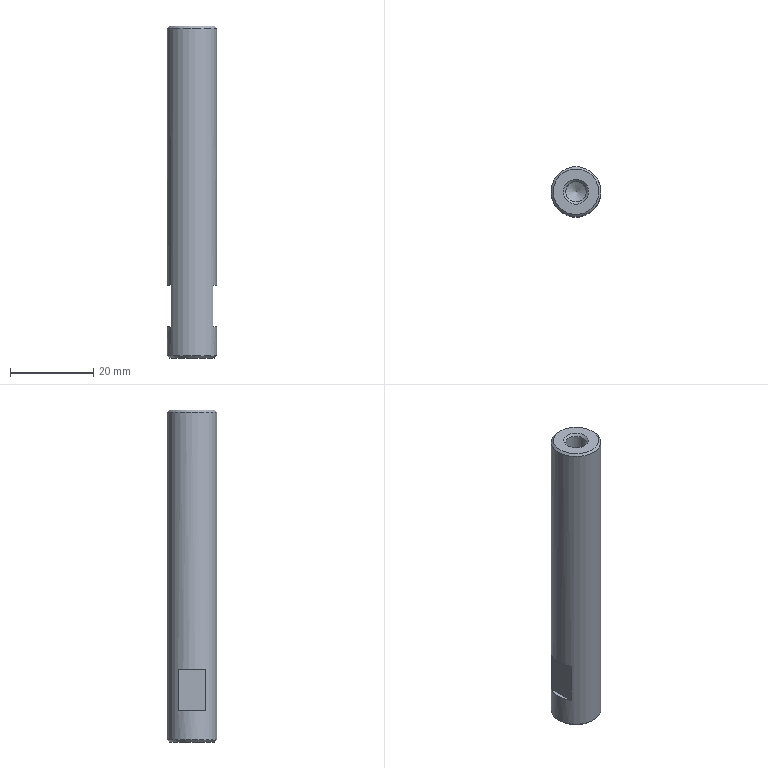Part | NX | features 5003_008_C-PETR12-80 2 | 1 solid | 17 faces | box 12 x 12 x 80 mm | volume 8295 mm3 | plane 8 | cone 6 | cylinder 3 | commonest cylinder face diameters 4.917 x2 12 x1
STEP:
#1=CARTESIAN_POINT('',(135.525,-262.,-324.5));
#2=VERTEX_POINT('',#1);
#3=CARTESIAN_POINT('',(141.525,-262.,-324.5));
#4=DIRECTION('',(0.,0.,1.));
#5=DIRECTION('',(-1.,0.,0.));
#6=AXIS2_PLACEMENT_3D('',#3,#4,#5);
#7=CIRCLE('',#6,6.);
#8=EDGE_CURVE('',#2,#2,#7,.T.);
#9=ORIENTED_EDGE('',*,*,#8,.T.);
#10=EDGE_LOOP('',(#9));
#11=FACE_BOUND('',#10,.T.);
#12=CARTESIAN_POINT('',(147.525,-262.,-245.5));
#13=VERTEX_POINT('',#12);
#14=CARTESIAN_POINT('',(141.525,-262.,-245.5));
#15=DIRECTION('',(0.,0.,-1.));
#16=DIRECTION('',(1.,0.,0.));
#17=AXIS2_PLACEMENT_3D('',#14,#15,#16);
#18=CIRCLE('',#17,6.);
#19=EDGE_CURVE('',#13,#13,#18,.T.);
#20=ORIENTED_EDGE('',*,*,#19,.T.);
#21=EDGE_LOOP('',(#20));
#22=FACE_BOUND('',#21,.T.);
#23=CARTESIAN_POINT('',(136.525,-265.317,-307.5));
#24=VERTEX_POINT('',#23);
#25=CARTESIAN_POINT('',(136.525,-258.683,-307.5));
#26=VERTEX_POINT('',#25);
#27=CARTESIAN_POINT('',(141.525,-262.,-307.5));
#28=DIRECTION('',(0.,0.,-1.));
#29=DIRECTION('',(1.,0.,0.));
#30=AXIS2_PLACEMENT_3D('',#27,#28,#29);
#31=CIRCLE('',#30,6.);
#32=EDGE_CURVE('',#24,#26,#31,.T.);
#33=ORIENTED_EDGE('',*,*,#32,.F.);
#34=CARTESIAN_POINT('',(136.525,-265.317,-317.5));
#35=VERTEX_POINT('',#34);
#36=CARTESIAN_POINT('',(136.525,-265.317,-325.));
#37=DIRECTION('',(0.,0.,-1.));
#38=VECTOR('',#37,1000.);
#39=LINE('',#36,#38);
#40=EDGE_CURVE('',#35,#24,#39,.F.);
#41=ORIENTED_EDGE('',*,*,#40,.F.);
#42=CARTESIAN_POINT('',(136.525,-258.683,-317.5));
#43=VERTEX_POINT('',#42);
#44=CARTESIAN_POINT('',(141.525,-262.,-317.5));
#45=DIRECTION('',(0.,0.,1.));
#46=DIRECTION('',(-1.,0.,0.));
#47=AXIS2_PLACEMENT_3D('',#44,#45,#46);
#48=CIRCLE('',#47,6.);
#49=EDGE_CURVE('',#43,#35,#48,.T.);
#50=ORIENTED_EDGE('',*,*,#49,.F.);
#51=CARTESIAN_POINT('',(136.525,-258.683,-325.));
#52=DIRECTION('',(0.,0.,-1.));
#53=VECTOR('',#52,1000.);
#54=LINE('',#51,#53);
#55=EDGE_CURVE('',#26,#43,#54,.T.);
#56=ORIENTED_EDGE('',*,*,#55,.F.);
#57=EDGE_LOOP('',(#33,#41,#50,#56));
#58=FACE_BOUND('',#57,.T.);
#59=CARTESIAN_POINT('',(146.525,-265.317,-307.5));
#60=VERTEX_POINT('',#59);
#61=CARTESIAN_POINT('',(146.525,-265.317,-317.5));
#62=VERTEX_POINT('',#61);
#63=CARTESIAN_POINT('',(146.525,-265.317,-325.));
#64=DIRECTION('',(0.,0.,-1.));
#65=VECTOR('',#64,1000.);
#66=LINE('',#63,#65);
#67=EDGE_CURVE('',#60,#62,#66,.T.);
#68=ORIENTED_EDGE('',*,*,#67,.F.);
#69=CARTESIAN_POINT('',(146.525,-258.683,-307.5));
#70=VERTEX_POINT('',#69);
#71=CARTESIAN_POINT('',(141.525,-262.,-307.5));
#72=DIRECTION('',(0.,0.,-1.));
#73=DIRECTION('',(1.,0.,0.));
#74=AXIS2_PLACEMENT_3D('',#71,#72,#73);
#75=CIRCLE('',#74,6.);
#76=EDGE_CURVE('',#70,#60,#75,.T.);
#77=ORIENTED_EDGE('',*,*,#76,.F.);
#78=CARTESIAN_POINT('',(146.525,-258.683,-317.5));
#79=VERTEX_POINT('',#78);
#80=CARTESIAN_POINT('',(146.525,-258.683,-325.));
#81=DIRECTION('',(0.,0.,-1.));
#82=VECTOR('',#81,1000.);
#83=LINE('',#80,#82);
#84=EDGE_CURVE('',#79,#70,#83,.F.);
#85=ORIENTED_EDGE('',*,*,#84,.F.);
#86=CARTESIAN_POINT('',(141.525,-262.,-317.5));
#87=DIRECTION('',(0.,0.,1.));
#88=DIRECTION('',(-1.,0.,0.));
#89=AXIS2_PLACEMENT_3D('',#86,#87,#88);
#90=CIRCLE('',#89,6.);
#91=EDGE_CURVE('',#62,#79,#90,.T.);
#92=ORIENTED_EDGE('',*,*,#91,.F.);
#93=EDGE_LOOP('',(#68,#77,#85,#92));
#94=FACE_BOUND('',#93,.T.);
#95=CARTESIAN_POINT('',(141.525,-262.,-325.));
#96=DIRECTION('',(0.,0.,-1.));
#97=DIRECTION('',(1.,0.,0.));
#98=AXIS2_PLACEMENT_3D('',#95,#96,#97);
#99=CYLINDRICAL_SURFACE('',#98,6.);
#100=ADVANCED_FACE('',(#11,#22,#58,#94),#99,.T.);
#101=CARTESIAN_POINT('',(138.517,-262.,-325.));
#102=VERTEX_POINT('',#101);
#103=CARTESIAN_POINT('',(141.525,-262.,-325.));
#104=DIRECTION('',(0.,0.,1.));
#105=DIRECTION('',(-1.,0.,0.));
#106=AXIS2_PLACEMENT_3D('',#103,#104,#105);
#107=CIRCLE('',#106,3.009);
#108=EDGE_CURVE('',#102,#102,#107,.T.);
#109=ORIENTED_EDGE('',*,*,#108,.T.);
#110=EDGE_LOOP('',(#109));
#111=FACE_BOUND('',#110,.T.);
#112=CARTESIAN_POINT('',(136.025,-262.,-325.));
#113=VERTEX_POINT('',#112);
#114=CARTESIAN_POINT('',(141.525,-262.,-325.));
#115=DIRECTION('',(0.,0.,1.));
#116=DIRECTION('',(-1.,0.,0.));
#117=AXIS2_PLACEMENT_3D('',#114,#115,#116);
#118=CIRCLE('',#117,5.5);
#119=EDGE_CURVE('',#113,#113,#118,.F.);
#120=ORIENTED_EDGE('',*,*,#119,.T.);
#121=EDGE_LOOP('',(#120));
#122=FACE_BOUND('',#121,.T.);
#123=CARTESIAN_POINT('',(141.525,-262.,-325.));
#124=DIRECTION('',(0.,0.,1.));
#125=DIRECTION('',(-1.,0.,0.));
#126=AXIS2_PLACEMENT_3D('',#123,#124,#125);
#127=PLANE('',#126);
#128=ADVANCED_FACE('',(#111,#122),#127,.F.);
#129=CARTESIAN_POINT('',(144.534,-262.,-245.));
#130=VERTEX_POINT('',#129);
#131=CARTESIAN_POINT('',(141.525,-262.,-245.));
#132=DIRECTION('',(0.,0.,-1.));
#133=DIRECTION('',(1.,0.,0.));
#134=AXIS2_PLACEMENT_3D('',#131,#132,#133);
#135=CIRCLE('',#134,3.009);
#136=EDGE_CURVE('',#130,#130,#135,.T.);
#137=ORIENTED_EDGE('',*,*,#136,.T.);
#138=EDGE_LOOP('',(#137));
#139=FACE_BOUND('',#138,.T.);
#140=CARTESIAN_POINT('',(147.025,-262.,-245.));
#141=VERTEX_POINT('',#140);
#142=CARTESIAN_POINT('',(141.525,-262.,-245.));
#143=DIRECTION('',(0.,0.,-1.));
#144=DIRECTION('',(1.,0.,0.));
#145=AXIS2_PLACEMENT_3D('',#142,#143,#144);
#146=CIRCLE('',#145,5.5);
#147=EDGE_CURVE('',#141,#141,#146,.F.);
#148=ORIENTED_EDGE('',*,*,#147,.T.);
#149=EDGE_LOOP('',(#148));
#150=FACE_BOUND('',#149,.T.);
#151=CARTESIAN_POINT('',(141.525,-262.,-245.));
#152=DIRECTION('',(0.,0.,-1.));
#153=DIRECTION('',(1.,0.,0.));
#154=AXIS2_PLACEMENT_3D('',#151,#152,#153);
#155=PLANE('',#154);
#156=ADVANCED_FACE('',(#139,#150),#155,.F.);
#157=ORIENTED_EDGE('',*,*,#49,.T.);
#158=CARTESIAN_POINT('',(136.525,-272.,-317.5));
#159=DIRECTION('',(0.,1.,0.));
#160=VECTOR('',#159,1000.);
#161=LINE('',#158,#160);
#162=EDGE_CURVE('',#35,#43,#161,.T.);
#163=ORIENTED_EDGE('',*,*,#162,.T.);
#164=EDGE_LOOP('',(#157,#163));
#165=FACE_BOUND('',#164,.T.);
#166=CARTESIAN_POINT('',(135.525,-272.,-317.5));
#167=DIRECTION('',(0.,0.,1.));
#168=DIRECTION('',(-1.,0.,0.));
#169=AXIS2_PLACEMENT_3D('',#166,#167,#168);
#170=PLANE('',#169);
#171=ADVANCED_FACE('',(#165),#170,.T.);
#172=ORIENTED_EDGE('',*,*,#55,.T.);
#173=ORIENTED_EDGE('',*,*,#162,.F.);
#174=ORIENTED_EDGE('',*,*,#40,.T.);
#175=CARTESIAN_POINT('',(136.525,-272.,-307.5));
#176=DIRECTION('',(0.,1.,0.));
#177=VECTOR('',#176,1000.);
#178=LINE('',#175,#177);
#179=EDGE_CURVE('',#24,#26,#178,.T.);
#180=ORIENTED_EDGE('',*,*,#179,.T.);
#181=EDGE_LOOP('',(#172,#173,#174,#180));
#182=FACE_BOUND('',#181,.T.);
#183=CARTESIAN_POINT('',(136.525,-272.,-317.5));
#184=DIRECTION('',(-1.,0.,0.));
#185=DIRECTION('',(0.,0.,-1.));
#186=AXIS2_PLACEMENT_3D('',#183,#184,#185);
#187=PLANE('',#186);
#188=ADVANCED_FACE('',(#182),#187,.T.);
#189=ORIENTED_EDGE('',*,*,#179,.F.);
#190=ORIENTED_EDGE('',*,*,#32,.T.);
#191=EDGE_LOOP('',(#189,#190));
#192=FACE_BOUND('',#191,.T.);
#193=CARTESIAN_POINT('',(135.525,-272.,-307.5));
#194=DIRECTION('',(0.,0.,-1.));
#195=DIRECTION('',(1.,0.,0.));
#196=AXIS2_PLACEMENT_3D('',#193,#194,#195);
#197=PLANE('',#196);
#198=ADVANCED_FACE('',(#192),#197,.T.);
#199=ORIENTED_EDGE('',*,*,#76,.T.);
#200=CARTESIAN_POINT('',(146.525,-272.,-307.5));
#201=DIRECTION('',(0.,1.,0.));
#202=VECTOR('',#201,1000.);
#203=LINE('',#200,#202);
#204=EDGE_CURVE('',#60,#70,#203,.T.);
#205=ORIENTED_EDGE('',*,*,#204,.T.);
#206=EDGE_LOOP('',(#199,#205));
#207=FACE_BOUND('',#206,.T.);
#208=CARTESIAN_POINT('',(147.525,-272.,-307.5));
#209=DIRECTION('',(0.,0.,-1.));
#210=DIRECTION('',(1.,0.,0.));
#211=AXIS2_PLACEMENT_3D('',#208,#209,#210);
#212=PLANE('',#211);
#213=ADVANCED_FACE('',(#207),#212,.T.);
#214=ORIENTED_EDGE('',*,*,#67,.T.);
#215=CARTESIAN_POINT('',(146.525,-272.,-317.5));
#216=DIRECTION('',(0.,1.,0.));
#217=VECTOR('',#216,1000.);
#218=LINE('',#215,#217);
#219=EDGE_CURVE('',#62,#79,#218,.T.);
#220=ORIENTED_EDGE('',*,*,#219,.T.);
#221=ORIENTED_EDGE('',*,*,#84,.T.);
#222=ORIENTED_EDGE('',*,*,#204,.F.);
#223=EDGE_LOOP('',(#214,#220,#221,#222));
#224=FACE_BOUND('',#223,.T.);
#225=CARTESIAN_POINT('',(146.525,-272.,-317.5));
#226=DIRECTION('',(1.,0.,0.));
#227=DIRECTION('',(0.,0.,1.));
#228=AXIS2_PLACEMENT_3D('',#225,#226,#227);
#229=PLANE('',#228);
#230=ADVANCED_FACE('',(#224),#229,.T.);
#231=ORIENTED_EDGE('',*,*,#219,.F.);
#232=ORIENTED_EDGE('',*,*,#91,.T.);
#233=EDGE_LOOP('',(#231,#232));
#234=FACE_BOUND('',#233,.T.);
#235=CARTESIAN_POINT('',(147.525,-272.,-317.5));
#236=DIRECTION('',(0.,0.,1.));
#237=DIRECTION('',(-1.,0.,0.));
#238=AXIS2_PLACEMENT_3D('',#235,#236,#237);
#239=PLANE('',#238);
#240=ADVANCED_FACE('',(#234),#239,.T.);
#241=ORIENTED_EDGE('',*,*,#8,.F.);
#242=EDGE_LOOP('',(#241));
#243=FACE_BOUND('',#242,.T.);
#244=ORIENTED_EDGE('',*,*,#119,.F.);
#245=EDGE_LOOP('',(#244));
#246=FACE_BOUND('',#245,.T.);
#247=CARTESIAN_POINT('',(141.525,-262.,-325.));
#248=DIRECTION('',(0.,0.,1.));
#249=DIRECTION('',(-1.,0.,0.));
#250=AXIS2_PLACEMENT_3D('',#247,#248,#249);
#251=CONICAL_SURFACE('',#250,5.5,0.7854);
#252=ADVANCED_FACE('',(#243,#246),#251,.T.);
#253=ORIENTED_EDGE('',*,*,#147,.F.);
#254=EDGE_LOOP('',(#253));
#255=FACE_BOUND('',#254,.T.);
#256=ORIENTED_EDGE('',*,*,#19,.F.);
#257=EDGE_LOOP('',(#256));
#258=FACE_BOUND('',#257,.T.);
#259=CARTESIAN_POINT('',(141.525,-262.,-245.5));
#260=DIRECTION('',(0.,0.,-1.));
#261=DIRECTION('',(1.,0.,0.));
#262=AXIS2_PLACEMENT_3D('',#259,#260,#261);
#263=CONICAL_SURFACE('',#262,6.,0.7854);
#264=ADVANCED_FACE('',(#255,#258),#263,.T.);
#265=CARTESIAN_POINT('',(141.525,-262.,-263.057));
#266=VERTEX_POINT('',#265);
#267=VERTEX_LOOP('',#266);
#268=FACE_BOUND('',#267,.T.);
#269=CARTESIAN_POINT('',(139.067,-262.,-261.58));
#270=VERTEX_POINT('',#269);
#271=CARTESIAN_POINT('',(141.525,-262.,-261.58));
#272=DIRECTION('',(0.,0.,1.));
#273=DIRECTION('',(-1.,0.,0.));
#274=AXIS2_PLACEMENT_3D('',#271,#272,#273);
#275=CIRCLE('',#274,2.458);
#276=EDGE_CURVE('',#270,#270,#275,.T.);
#277=ORIENTED_EDGE('',*,*,#276,.T.);
#278=EDGE_LOOP('',(#277));
#279=FACE_BOUND('',#278,.T.);
#280=CARTESIAN_POINT('',(141.525,-262.,-261.58));
#281=DIRECTION('',(0.,0.,1.));
#282=DIRECTION('',(-1.,0.,0.));
#283=AXIS2_PLACEMENT_3D('',#280,#281,#282);
#284=CONICAL_SURFACE('',#283,2.458,1.03);
#285=ADVANCED_FACE('',(#268,#279),#284,.F.);
#286=CARTESIAN_POINT('',(143.984,-262.,-245.55));
#287=VERTEX_POINT('',#286);
#288=CARTESIAN_POINT('',(141.525,-262.,-245.55));
#289=DIRECTION('',(0.,0.,-1.));
#290=DIRECTION('',(1.,0.,0.));
#291=AXIS2_PLACEMENT_3D('',#288,#289,#290);
#292=CIRCLE('',#291,2.458);
#293=EDGE_CURVE('',#287,#287,#292,.F.);
#294=ORIENTED_EDGE('',*,*,#293,.T.);
#295=EDGE_LOOP('',(#294));
#296=FACE_BOUND('',#295,.T.);
#297=ORIENTED_EDGE('',*,*,#276,.F.);
#298=EDGE_LOOP('',(#297));
#299=FACE_BOUND('',#298,.T.);
#300=CARTESIAN_POINT('',(141.525,-262.,-245.));
#301=DIRECTION('',(0.,0.,1.));
#302=DIRECTION('',(-1.,0.,0.));
#303=AXIS2_PLACEMENT_3D('',#300,#301,#302);
#304=CYLINDRICAL_SURFACE('',#303,2.458);
#305=ADVANCED_FACE('',(#296,#299),#304,.F.);
#306=CARTESIAN_POINT('',(141.525,-262.,-306.943));
#307=VERTEX_POINT('',#306);
#308=VERTEX_LOOP('',#307);
#309=FACE_BOUND('',#308,.T.);
#310=CARTESIAN_POINT('',(143.984,-262.,-308.42));
#311=VERTEX_POINT('',#310);
#312=CARTESIAN_POINT('',(141.525,-262.,-308.42));
#313=DIRECTION('',(0.,0.,-1.));
#314=DIRECTION('',(1.,0.,0.));
#315=AXIS2_PLACEMENT_3D('',#312,#313,#314);
#316=CIRCLE('',#315,2.458);
#317=EDGE_CURVE('',#311,#311,#316,.T.);
#318=ORIENTED_EDGE('',*,*,#317,.T.);
#319=EDGE_LOOP('',(#318));
#320=FACE_BOUND('',#319,.T.);
#321=CARTESIAN_POINT('',(141.525,-262.,-308.42));
#322=DIRECTION('',(0.,0.,-1.));
#323=DIRECTION('',(1.,0.,0.));
#324=AXIS2_PLACEMENT_3D('',#321,#322,#323);
#325=CONICAL_SURFACE('',#324,2.458,1.03);
#326=ADVANCED_FACE('',(#309,#320),#325,.F.);
#327=CARTESIAN_POINT('',(139.067,-262.,-324.45));
#328=VERTEX_POINT('',#327);
#329=CARTESIAN_POINT('',(141.525,-262.,-324.45));
#330=DIRECTION('',(0.,0.,1.));
#331=DIRECTION('',(-1.,0.,0.));
#332=AXIS2_PLACEMENT_3D('',#329,#330,#331);
#333=CIRCLE('',#332,2.458);
#334=EDGE_CURVE('',#328,#328,#333,.F.);
#335=ORIENTED_EDGE('',*,*,#334,.T.);
#336=EDGE_LOOP('',(#335));
#337=FACE_BOUND('',#336,.T.);
#338=ORIENTED_EDGE('',*,*,#317,.F.);
#339=EDGE_LOOP('',(#338));
#340=FACE_BOUND('',#339,.T.);
#341=CARTESIAN_POINT('',(141.525,-262.,-325.));
#342=DIRECTION('',(0.,0.,-1.));
#343=DIRECTION('',(1.,0.,0.));
#344=AXIS2_PLACEMENT_3D('',#341,#342,#343);
#345=CYLINDRICAL_SURFACE('',#344,2.458);
#346=ADVANCED_FACE('',(#337,#340),#345,.F.);
#347=ORIENTED_EDGE('',*,*,#108,.F.);
#348=EDGE_LOOP('',(#347));
#349=FACE_BOUND('',#348,.T.);
#350=ORIENTED_EDGE('',*,*,#334,.F.);
#351=EDGE_LOOP('',(#350));
#352=FACE_BOUND('',#351,.T.);
#353=CARTESIAN_POINT('',(141.525,-262.,-324.45));
#354=DIRECTION('',(0.,0.,-1.));
#355=DIRECTION('',(1.,0.,0.));
#356=AXIS2_PLACEMENT_3D('',#353,#354,#355);
#357=CONICAL_SURFACE('',#356,2.458,0.7854);
#358=ADVANCED_FACE('',(#349,#352),#357,.F.);
#359=ORIENTED_EDGE('',*,*,#136,.F.);
#360=EDGE_LOOP('',(#359));
#361=FACE_BOUND('',#360,.T.);
#362=ORIENTED_EDGE('',*,*,#293,.F.);
#363=EDGE_LOOP('',(#362));
#364=FACE_BOUND('',#363,.T.);
#365=CARTESIAN_POINT('',(141.525,-262.,-245.55));
#366=DIRECTION('',(0.,0.,1.));
#367=DIRECTION('',(-1.,0.,0.));
#368=AXIS2_PLACEMENT_3D('',#365,#366,#367);
#369=CONICAL_SURFACE('',#368,2.458,0.7854);
#370=ADVANCED_FACE('',(#361,#364),#369,.F.);
#371=CLOSED_SHELL('',(#100,#128,#156,#171,#188,#198,#213,#230,#240,#252,#264,#285,#305,#326,#346,#358,#370));
#372=MANIFOLD_SOLID_BREP('',#371);
#373=(LENGTH_UNIT()NAMED_UNIT(*)SI_UNIT(.MILLI.,.METRE.));
#374=UNCERTAINTY_MEASURE_WITH_UNIT(LENGTH_MEASURE(0.00001),#373,'','');
#375=(NAMED_UNIT(*)PLANE_ANGLE_UNIT()SI_UNIT($,.RADIAN.));
#376=(NAMED_UNIT(*)SI_UNIT($,.STERADIAN.)SOLID_ANGLE_UNIT());
#377=(GEOMETRIC_REPRESENTATION_CONTEXT(3)GLOBAL_UNCERTAINTY_ASSIGNED_CONTEXT((#374))GLOBAL_UNIT_ASSIGNED_CONTEXT((#373,#375,#376))REPRESENTATION_CONTEXT('',''));
#378=ADVANCED_BREP_SHAPE_REPRESENTATION('',(#372),#377);